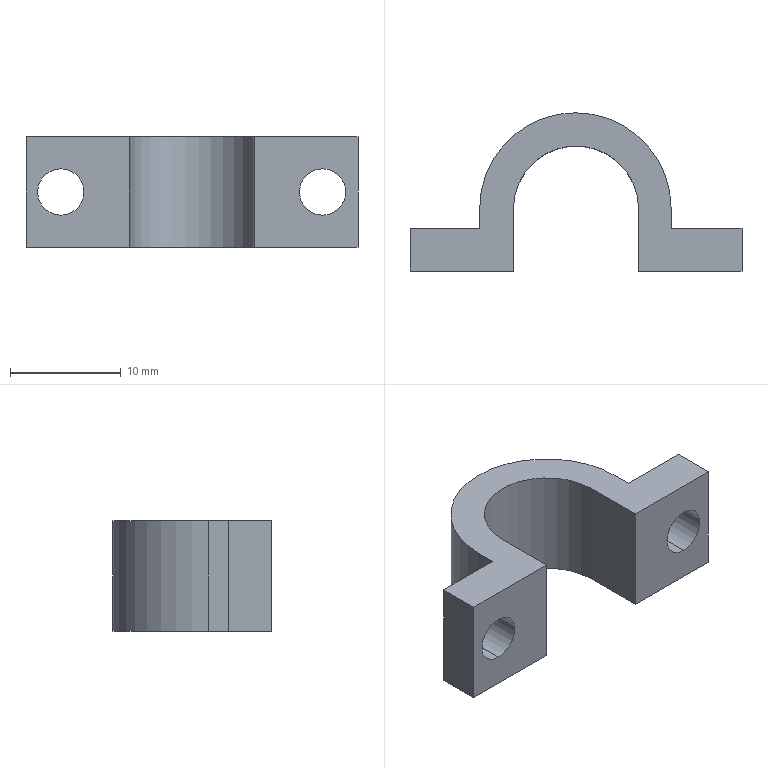Part | SolidWorks | features Cut 1, Extrusion 1 | 1 solid | 18 faces | box 30 x 14.3 x 10 mm | volume 1395 mm3 | plane 12 | cylinder 6 | commonest cylinder face diameters 4.2 x4 11.3 x1 17.3 x1
STEP:
#1=CARTESIAN_POINT('',(11.852,1.335,2.9));
#2=VERTEX_POINT('',#1);
#3=CARTESIAN_POINT('',(11.852,1.335,7.1));
#4=VERTEX_POINT('',#3);
#5=CARTESIAN_POINT('',(11.852,1.335,5.));
#6=DIRECTION('',(0.,1.,0.));
#7=DIRECTION('',(0.,0.,1.));
#8=AXIS2_PLACEMENT_3D('',#5,#6,#7);
#9=CIRCLE('',#8,2.1);
#10=EDGE_CURVE('',#2,#4,#9,.T.);
#11=ORIENTED_EDGE('',*,*,#10,.F.);
#12=CARTESIAN_POINT('',(11.852,5.185,2.9));
#13=VERTEX_POINT('',#12);
#14=CARTESIAN_POINT('',(11.852,-18.455,2.9));
#15=DIRECTION('',(0.,1.,0.));
#16=VECTOR('',#15,1000.);
#17=LINE('',#14,#16);
#18=EDGE_CURVE('',#2,#13,#17,.T.);
#19=ORIENTED_EDGE('',*,*,#18,.T.);
#20=CARTESIAN_POINT('',(11.852,5.185,7.1));
#21=VERTEX_POINT('',#20);
#22=CARTESIAN_POINT('',(11.852,5.185,5.));
#23=DIRECTION('',(0.,1.,0.));
#24=DIRECTION('',(0.,0.,1.));
#25=AXIS2_PLACEMENT_3D('',#22,#23,#24);
#26=CIRCLE('',#25,2.1);
#27=EDGE_CURVE('',#13,#21,#26,.T.);
#28=ORIENTED_EDGE('',*,*,#27,.T.);
#29=CARTESIAN_POINT('',(11.852,-18.455,7.1));
#30=DIRECTION('',(0.,1.,0.));
#31=VECTOR('',#30,1000.);
#32=LINE('',#29,#31);
#33=EDGE_CURVE('',#4,#21,#32,.T.);
#34=ORIENTED_EDGE('',*,*,#33,.F.);
#35=EDGE_LOOP('',(#11,#19,#28,#34));
#36=FACE_OUTER_BOUND('',#35,.T.);
#37=CARTESIAN_POINT('',(11.852,-18.455,5.));
#38=DIRECTION('',(0.,1.,0.));
#39=DIRECTION('',(0.,0.,1.));
#40=AXIS2_PLACEMENT_3D('',#37,#38,#39);
#41=CYLINDRICAL_SURFACE('',#40,2.1);
#42=ADVANCED_FACE('',(#36),#41,.F.);
#43=CARTESIAN_POINT('',(-11.798,1.335,2.9));
#44=VERTEX_POINT('',#43);
#45=CARTESIAN_POINT('',(-11.798,1.335,7.1));
#46=VERTEX_POINT('',#45);
#47=CARTESIAN_POINT('',(-11.798,1.335,5.));
#48=DIRECTION('',(0.,1.,0.));
#49=DIRECTION('',(0.,0.,1.));
#50=AXIS2_PLACEMENT_3D('',#47,#48,#49);
#51=CIRCLE('',#50,2.1);
#52=EDGE_CURVE('',#44,#46,#51,.T.);
#53=ORIENTED_EDGE('',*,*,#52,.F.);
#54=CARTESIAN_POINT('',(-11.798,5.185,2.9));
#55=VERTEX_POINT('',#54);
#56=CARTESIAN_POINT('',(-11.798,-18.455,2.9));
#57=DIRECTION('',(0.,1.,0.));
#58=VECTOR('',#57,1000.);
#59=LINE('',#56,#58);
#60=EDGE_CURVE('',#44,#55,#59,.T.);
#61=ORIENTED_EDGE('',*,*,#60,.T.);
#62=CARTESIAN_POINT('',(-11.798,5.185,7.1));
#63=VERTEX_POINT('',#62);
#64=CARTESIAN_POINT('',(-11.798,5.185,5.));
#65=DIRECTION('',(0.,1.,0.));
#66=DIRECTION('',(0.,0.,1.));
#67=AXIS2_PLACEMENT_3D('',#64,#65,#66);
#68=CIRCLE('',#67,2.1);
#69=EDGE_CURVE('',#55,#63,#68,.T.);
#70=ORIENTED_EDGE('',*,*,#69,.T.);
#71=CARTESIAN_POINT('',(-11.798,-18.455,7.1));
#72=DIRECTION('',(0.,1.,0.));
#73=VECTOR('',#72,1000.);
#74=LINE('',#71,#73);
#75=EDGE_CURVE('',#46,#63,#74,.T.);
#76=ORIENTED_EDGE('',*,*,#75,.F.);
#77=EDGE_LOOP('',(#53,#61,#70,#76));
#78=FACE_OUTER_BOUND('',#77,.T.);
#79=CARTESIAN_POINT('',(-11.798,-18.455,5.));
#80=DIRECTION('',(0.,1.,0.));
#81=DIRECTION('',(0.,0.,1.));
#82=AXIS2_PLACEMENT_3D('',#79,#80,#81);
#83=CYLINDRICAL_SURFACE('',#82,2.1);
#84=ADVANCED_FACE('',(#78),#83,.F.);
#85=CARTESIAN_POINT('',(-14.947,5.185,0.));
#86=VERTEX_POINT('',#85);
#87=CARTESIAN_POINT('',(-14.947,1.335,0.));
#88=VERTEX_POINT('',#87);
#89=CARTESIAN_POINT('',(-14.947,5.185,0.));
#90=DIRECTION('',(0.,-1.,0.));
#91=VECTOR('',#90,1000.);
#92=LINE('',#89,#91);
#93=EDGE_CURVE('',#86,#88,#92,.T.);
#94=ORIENTED_EDGE('',*,*,#93,.T.);
#95=CARTESIAN_POINT('',(-14.947,1.335,10.));
#96=VERTEX_POINT('',#95);
#97=CARTESIAN_POINT('',(-14.947,1.335,10.));
#98=DIRECTION('',(0.,0.,-1.));
#99=VECTOR('',#98,1000.);
#100=LINE('',#97,#99);
#101=EDGE_CURVE('',#96,#88,#100,.T.);
#102=ORIENTED_EDGE('',*,*,#101,.F.);
#103=CARTESIAN_POINT('',(-14.947,5.185,10.));
#104=VERTEX_POINT('',#103);
#105=CARTESIAN_POINT('',(-14.947,5.185,10.));
#106=DIRECTION('',(0.,-1.,0.));
#107=VECTOR('',#106,1000.);
#108=LINE('',#105,#107);
#109=EDGE_CURVE('',#104,#96,#108,.T.);
#110=ORIENTED_EDGE('',*,*,#109,.F.);
#111=CARTESIAN_POINT('',(-14.947,5.185,10.));
#112=DIRECTION('',(0.,0.,-1.));
#113=VECTOR('',#112,1000.);
#114=LINE('',#111,#113);
#115=EDGE_CURVE('',#104,#86,#114,.T.);
#116=ORIENTED_EDGE('',*,*,#115,.T.);
#117=EDGE_LOOP('',(#94,#102,#110,#116));
#118=FACE_OUTER_BOUND('',#117,.T.);
#119=CARTESIAN_POINT('',(-14.947,5.185,10.));
#120=DIRECTION('',(1.,0.,0.));
#121=DIRECTION('',(0.,0.,-1.));
#122=AXIS2_PLACEMENT_3D('',#119,#120,#121);
#123=PLANE('',#122);
#124=ADVANCED_FACE('',(#118),#123,.F.);
#125=CARTESIAN_POINT('',(-11.798,1.335,5.));
#126=DIRECTION('',(0.,1.,0.));
#127=DIRECTION('',(0.,0.,1.));
#128=AXIS2_PLACEMENT_3D('',#125,#126,#127);
#129=CIRCLE('',#128,2.1);
#130=EDGE_CURVE('',#46,#44,#129,.T.);
#131=ORIENTED_EDGE('',*,*,#130,.T.);
#132=ORIENTED_EDGE('',*,*,#52,.T.);
#133=EDGE_LOOP('',(#131,#132));
#134=FACE_BOUND('',#133,.T.);
#135=CARTESIAN_POINT('',(-5.597,1.335,0.));
#136=VERTEX_POINT('',#135);
#137=CARTESIAN_POINT('',(-14.947,1.335,0.));
#138=DIRECTION('',(1.,0.,0.));
#139=VECTOR('',#138,1000.);
#140=LINE('',#137,#139);
#141=EDGE_CURVE('',#88,#136,#140,.T.);
#142=ORIENTED_EDGE('',*,*,#141,.T.);
#143=CARTESIAN_POINT('',(-5.597,1.335,10.));
#144=VERTEX_POINT('',#143);
#145=CARTESIAN_POINT('',(-5.597,1.335,10.));
#146=DIRECTION('',(0.,0.,-1.));
#147=VECTOR('',#146,1000.);
#148=LINE('',#145,#147);
#149=EDGE_CURVE('',#144,#136,#148,.T.);
#150=ORIENTED_EDGE('',*,*,#149,.F.);
#151=CARTESIAN_POINT('',(-14.947,1.335,10.));
#152=DIRECTION('',(1.,0.,0.));
#153=VECTOR('',#152,1000.);
#154=LINE('',#151,#153);
#155=EDGE_CURVE('',#96,#144,#154,.T.);
#156=ORIENTED_EDGE('',*,*,#155,.F.);
#157=ORIENTED_EDGE('',*,*,#101,.T.);
#158=EDGE_LOOP('',(#142,#150,#156,#157));
#159=FACE_OUTER_BOUND('',#158,.T.);
#160=CARTESIAN_POINT('',(-14.947,1.335,10.));
#161=DIRECTION('',(0.,1.,0.));
#162=DIRECTION('',(0.,0.,1.));
#163=AXIS2_PLACEMENT_3D('',#160,#161,#162);
#164=PLANE('',#163);
#165=ADVANCED_FACE('',(#134,#159),#164,.F.);
#166=CARTESIAN_POINT('',(-5.597,6.985,0.));
#167=VERTEX_POINT('',#166);
#168=CARTESIAN_POINT('',(-5.597,5.185,0.));
#169=DIRECTION('',(0.,1.,0.));
#170=VECTOR('',#169,1000.);
#171=LINE('',#168,#170);
#172=EDGE_CURVE('',#136,#167,#171,.T.);
#173=ORIENTED_EDGE('',*,*,#172,.T.);
#174=CARTESIAN_POINT('',(-5.597,6.985,10.));
#175=VERTEX_POINT('',#174);
#176=CARTESIAN_POINT('',(-5.597,6.985,10.));
#177=DIRECTION('',(0.,0.,-1.));
#178=VECTOR('',#177,1000.);
#179=LINE('',#176,#178);
#180=EDGE_CURVE('',#175,#167,#179,.T.);
#181=ORIENTED_EDGE('',*,*,#180,.F.);
#182=CARTESIAN_POINT('',(-5.597,5.185,10.));
#183=DIRECTION('',(0.,1.,0.));
#184=VECTOR('',#183,1000.);
#185=LINE('',#182,#184);
#186=EDGE_CURVE('',#144,#175,#185,.T.);
#187=ORIENTED_EDGE('',*,*,#186,.F.);
#188=ORIENTED_EDGE('',*,*,#149,.T.);
#189=EDGE_LOOP('',(#173,#181,#187,#188));
#190=FACE_OUTER_BOUND('',#189,.T.);
#191=CARTESIAN_POINT('',(-5.597,5.185,10.));
#192=DIRECTION('',(-1.,0.,0.));
#193=DIRECTION('',(0.,0.,1.));
#194=AXIS2_PLACEMENT_3D('',#191,#192,#193);
#195=PLANE('',#194);
#196=ADVANCED_FACE('',(#190),#195,.F.);
#197=CARTESIAN_POINT('',(5.703,6.985,0.));
#198=VERTEX_POINT('',#197);
#199=CARTESIAN_POINT('',(0.05334,6.985,0.));
#200=DIRECTION('',(0.,0.,-1.));
#201=DIRECTION('',(1.,0.,0.));
#202=AXIS2_PLACEMENT_3D('',#199,#200,#201);
#203=CIRCLE('',#202,5.65);
#204=EDGE_CURVE('',#167,#198,#203,.T.);
#205=ORIENTED_EDGE('',*,*,#204,.T.);
#206=CARTESIAN_POINT('',(5.703,6.985,10.));
#207=VERTEX_POINT('',#206);
#208=CARTESIAN_POINT('',(5.703,6.985,10.));
#209=DIRECTION('',(0.,0.,-1.));
#210=VECTOR('',#209,1000.);
#211=LINE('',#208,#210);
#212=EDGE_CURVE('',#207,#198,#211,.T.);
#213=ORIENTED_EDGE('',*,*,#212,.F.);
#214=CARTESIAN_POINT('',(0.05334,6.985,10.));
#215=DIRECTION('',(0.,0.,-1.));
#216=DIRECTION('',(1.,0.,0.));
#217=AXIS2_PLACEMENT_3D('',#214,#215,#216);
#218=CIRCLE('',#217,5.65);
#219=EDGE_CURVE('',#175,#207,#218,.T.);
#220=ORIENTED_EDGE('',*,*,#219,.F.);
#221=ORIENTED_EDGE('',*,*,#180,.T.);
#222=EDGE_LOOP('',(#205,#213,#220,#221));
#223=FACE_OUTER_BOUND('',#222,.T.);
#224=CARTESIAN_POINT('',(0.05334,6.985,10.));
#225=DIRECTION('',(0.,0.,-1.));
#226=DIRECTION('',(-1.,0.,0.));
#227=AXIS2_PLACEMENT_3D('',#224,#225,#226);
#228=CYLINDRICAL_SURFACE('',#227,5.65);
#229=ADVANCED_FACE('',(#223),#228,.F.);
#230=CARTESIAN_POINT('',(5.703,1.335,0.));
#231=VERTEX_POINT('',#230);
#232=CARTESIAN_POINT('',(5.703,5.185,0.));
#233=DIRECTION('',(0.,-1.,0.));
#234=VECTOR('',#233,1000.);
#235=LINE('',#232,#234);
#236=EDGE_CURVE('',#198,#231,#235,.T.);
#237=ORIENTED_EDGE('',*,*,#236,.T.);
#238=CARTESIAN_POINT('',(5.703,1.335,10.));
#239=VERTEX_POINT('',#238);
#240=CARTESIAN_POINT('',(5.703,1.335,10.));
#241=DIRECTION('',(0.,0.,-1.));
#242=VECTOR('',#241,1000.);
#243=LINE('',#240,#242);
#244=EDGE_CURVE('',#239,#231,#243,.T.);
#245=ORIENTED_EDGE('',*,*,#244,.F.);
#246=CARTESIAN_POINT('',(5.703,6.985,10.));
#247=DIRECTION('',(0.,-1.,0.));
#248=VECTOR('',#247,1000.);
#249=LINE('',#246,#248);
#250=EDGE_CURVE('',#207,#239,#249,.T.);
#251=ORIENTED_EDGE('',*,*,#250,.F.);
#252=ORIENTED_EDGE('',*,*,#212,.T.);
#253=EDGE_LOOP('',(#237,#245,#251,#252));
#254=FACE_OUTER_BOUND('',#253,.T.);
#255=CARTESIAN_POINT('',(5.703,5.185,10.));
#256=DIRECTION('',(1.,0.,0.));
#257=DIRECTION('',(0.,1.,0.));
#258=AXIS2_PLACEMENT_3D('',#255,#256,#257);
#259=PLANE('',#258);
#260=ADVANCED_FACE('',(#254),#259,.F.);
#261=CARTESIAN_POINT('',(11.852,1.335,5.));
#262=DIRECTION('',(0.,1.,0.));
#263=DIRECTION('',(0.,0.,1.));
#264=AXIS2_PLACEMENT_3D('',#261,#262,#263);
#265=CIRCLE('',#264,2.1);
#266=EDGE_CURVE('',#4,#2,#265,.T.);
#267=ORIENTED_EDGE('',*,*,#266,.T.);
#268=ORIENTED_EDGE('',*,*,#10,.T.);
#269=EDGE_LOOP('',(#267,#268));
#270=FACE_BOUND('',#269,.T.);
#271=CARTESIAN_POINT('',(15.053,1.335,0.));
#272=VERTEX_POINT('',#271);
#273=CARTESIAN_POINT('',(5.703,1.335,0.));
#274=DIRECTION('',(1.,0.,0.));
#275=VECTOR('',#274,1000.);
#276=LINE('',#273,#275);
#277=EDGE_CURVE('',#231,#272,#276,.T.);
#278=ORIENTED_EDGE('',*,*,#277,.T.);
#279=CARTESIAN_POINT('',(15.053,1.335,10.));
#280=VERTEX_POINT('',#279);
#281=CARTESIAN_POINT('',(15.053,1.335,10.));
#282=DIRECTION('',(0.,0.,-1.));
#283=VECTOR('',#282,1000.);
#284=LINE('',#281,#283);
#285=EDGE_CURVE('',#280,#272,#284,.T.);
#286=ORIENTED_EDGE('',*,*,#285,.F.);
#287=CARTESIAN_POINT('',(5.703,1.335,10.));
#288=DIRECTION('',(1.,0.,0.));
#289=VECTOR('',#288,1000.);
#290=LINE('',#287,#289);
#291=EDGE_CURVE('',#239,#280,#290,.T.);
#292=ORIENTED_EDGE('',*,*,#291,.F.);
#293=ORIENTED_EDGE('',*,*,#244,.T.);
#294=EDGE_LOOP('',(#278,#286,#292,#293));
#295=FACE_OUTER_BOUND('',#294,.T.);
#296=CARTESIAN_POINT('',(5.703,1.335,10.));
#297=DIRECTION('',(0.,1.,0.));
#298=DIRECTION('',(0.,0.,1.));
#299=AXIS2_PLACEMENT_3D('',#296,#297,#298);
#300=PLANE('',#299);
#301=ADVANCED_FACE('',(#270,#295),#300,.F.);
#302=CARTESIAN_POINT('',(15.053,5.185,0.));
#303=VERTEX_POINT('',#302);
#304=CARTESIAN_POINT('',(15.053,5.185,0.));
#305=DIRECTION('',(0.,1.,0.));
#306=VECTOR('',#305,1000.);
#307=LINE('',#304,#306);
#308=EDGE_CURVE('',#272,#303,#307,.T.);
#309=ORIENTED_EDGE('',*,*,#308,.T.);
#310=CARTESIAN_POINT('',(15.053,5.185,10.));
#311=VERTEX_POINT('',#310);
#312=CARTESIAN_POINT('',(15.053,5.185,10.));
#313=DIRECTION('',(0.,0.,-1.));
#314=VECTOR('',#313,1000.);
#315=LINE('',#312,#314);
#316=EDGE_CURVE('',#311,#303,#315,.T.);
#317=ORIENTED_EDGE('',*,*,#316,.F.);
#318=CARTESIAN_POINT('',(15.053,5.185,10.));
#319=DIRECTION('',(0.,1.,0.));
#320=VECTOR('',#319,1000.);
#321=LINE('',#318,#320);
#322=EDGE_CURVE('',#280,#311,#321,.T.);
#323=ORIENTED_EDGE('',*,*,#322,.F.);
#324=ORIENTED_EDGE('',*,*,#285,.T.);
#325=EDGE_LOOP('',(#309,#317,#323,#324));
#326=FACE_OUTER_BOUND('',#325,.T.);
#327=CARTESIAN_POINT('',(15.053,5.185,10.));
#328=DIRECTION('',(-1.,0.,0.));
#329=DIRECTION('',(0.,-1.,0.));
#330=AXIS2_PLACEMENT_3D('',#327,#328,#329);
#331=PLANE('',#330);
#332=ADVANCED_FACE('',(#326),#331,.F.);
#333=CARTESIAN_POINT('',(11.852,5.185,5.));
#334=DIRECTION('',(0.,1.,0.));
#335=DIRECTION('',(0.,0.,1.));
#336=AXIS2_PLACEMENT_3D('',#333,#334,#335);
#337=CIRCLE('',#336,2.1);
#338=EDGE_CURVE('',#21,#13,#337,.T.);
#339=ORIENTED_EDGE('',*,*,#338,.F.);
#340=ORIENTED_EDGE('',*,*,#27,.F.);
#341=EDGE_LOOP('',(#339,#340));
#342=FACE_BOUND('',#341,.T.);
#343=CARTESIAN_POINT('',(8.65,5.185,0.));
#344=VERTEX_POINT('',#343);
#345=CARTESIAN_POINT('',(8.65,5.185,0.));
#346=DIRECTION('',(-1.,0.,0.));
#347=VECTOR('',#346,1000.);
#348=LINE('',#345,#347);
#349=EDGE_CURVE('',#303,#344,#348,.T.);
#350=ORIENTED_EDGE('',*,*,#349,.T.);
#351=CARTESIAN_POINT('',(8.65,5.185,10.));
#352=VERTEX_POINT('',#351);
#353=CARTESIAN_POINT('',(8.65,5.185,10.));
#354=DIRECTION('',(0.,0.,-1.));
#355=VECTOR('',#354,1000.);
#356=LINE('',#353,#355);
#357=EDGE_CURVE('',#352,#344,#356,.T.);
#358=ORIENTED_EDGE('',*,*,#357,.F.);
#359=CARTESIAN_POINT('',(8.65,5.185,10.));
#360=DIRECTION('',(-1.,0.,0.));
#361=VECTOR('',#360,1000.);
#362=LINE('',#359,#361);
#363=EDGE_CURVE('',#311,#352,#362,.T.);
#364=ORIENTED_EDGE('',*,*,#363,.F.);
#365=ORIENTED_EDGE('',*,*,#316,.T.);
#366=EDGE_LOOP('',(#350,#358,#364,#365));
#367=FACE_OUTER_BOUND('',#366,.T.);
#368=CARTESIAN_POINT('',(8.65,5.185,10.));
#369=DIRECTION('',(0.,-1.,0.));
#370=DIRECTION('',(0.,0.,-1.));
#371=AXIS2_PLACEMENT_3D('',#368,#369,#370);
#372=PLANE('',#371);
#373=ADVANCED_FACE('',(#342,#367),#372,.F.);
#374=CARTESIAN_POINT('',(8.65,6.985,0.));
#375=VERTEX_POINT('',#374);
#376=CARTESIAN_POINT('',(8.65,6.985,0.));
#377=DIRECTION('',(0.,1.,0.));
#378=VECTOR('',#377,1000.);
#379=LINE('',#376,#378);
#380=EDGE_CURVE('',#344,#375,#379,.T.);
#381=ORIENTED_EDGE('',*,*,#380,.T.);
#382=CARTESIAN_POINT('',(8.65,6.985,10.));
#383=VERTEX_POINT('',#382);
#384=CARTESIAN_POINT('',(8.65,6.985,10.));
#385=DIRECTION('',(0.,0.,-1.));
#386=VECTOR('',#385,1000.);
#387=LINE('',#384,#386);
#388=EDGE_CURVE('',#383,#375,#387,.T.);
#389=ORIENTED_EDGE('',*,*,#388,.F.);
#390=CARTESIAN_POINT('',(8.65,6.985,10.));
#391=DIRECTION('',(0.,1.,0.));
#392=VECTOR('',#391,1000.);
#393=LINE('',#390,#392);
#394=EDGE_CURVE('',#352,#383,#393,.T.);
#395=ORIENTED_EDGE('',*,*,#394,.F.);
#396=ORIENTED_EDGE('',*,*,#357,.T.);
#397=EDGE_LOOP('',(#381,#389,#395,#396));
#398=FACE_OUTER_BOUND('',#397,.T.);
#399=CARTESIAN_POINT('',(8.65,6.985,10.));
#400=DIRECTION('',(-1.,0.,0.));
#401=DIRECTION('',(0.,0.,1.));
#402=AXIS2_PLACEMENT_3D('',#399,#400,#401);
#403=PLANE('',#402);
#404=ADVANCED_FACE('',(#398),#403,.F.);
#405=CARTESIAN_POINT('',(-8.65,6.985,0.));
#406=VERTEX_POINT('',#405);
#407=CARTESIAN_POINT('',(0.,6.985,0.));
#408=DIRECTION('',(0.,0.,1.));
#409=DIRECTION('',(1.,0.,0.));
#410=AXIS2_PLACEMENT_3D('',#407,#408,#409);
#411=CIRCLE('',#410,8.65);
#412=EDGE_CURVE('',#375,#406,#411,.T.);
#413=ORIENTED_EDGE('',*,*,#412,.T.);
#414=CARTESIAN_POINT('',(-8.65,6.985,10.));
#415=VERTEX_POINT('',#414);
#416=CARTESIAN_POINT('',(-8.65,6.985,10.));
#417=DIRECTION('',(0.,0.,-1.));
#418=VECTOR('',#417,1000.);
#419=LINE('',#416,#418);
#420=EDGE_CURVE('',#415,#406,#419,.T.);
#421=ORIENTED_EDGE('',*,*,#420,.F.);
#422=CARTESIAN_POINT('',(0.,6.985,10.));
#423=DIRECTION('',(0.,0.,1.));
#424=DIRECTION('',(1.,0.,0.));
#425=AXIS2_PLACEMENT_3D('',#422,#423,#424);
#426=CIRCLE('',#425,8.65);
#427=EDGE_CURVE('',#383,#415,#426,.T.);
#428=ORIENTED_EDGE('',*,*,#427,.F.);
#429=ORIENTED_EDGE('',*,*,#388,.T.);
#430=EDGE_LOOP('',(#413,#421,#428,#429));
#431=FACE_OUTER_BOUND('',#430,.T.);
#432=CARTESIAN_POINT('',(0.,6.985,10.));
#433=DIRECTION('',(0.,0.,-1.));
#434=DIRECTION('',(-1.,0.,0.));
#435=AXIS2_PLACEMENT_3D('',#432,#433,#434);
#436=CYLINDRICAL_SURFACE('',#435,8.65);
#437=ADVANCED_FACE('',(#431),#436,.T.);
#438=CARTESIAN_POINT('',(-8.65,5.185,0.));
#439=VERTEX_POINT('',#438);
#440=CARTESIAN_POINT('',(-8.65,6.985,0.));
#441=DIRECTION('',(0.,-1.,0.));
#442=VECTOR('',#441,1000.);
#443=LINE('',#440,#442);
#444=EDGE_CURVE('',#406,#439,#443,.T.);
#445=ORIENTED_EDGE('',*,*,#444,.T.);
#446=CARTESIAN_POINT('',(-8.65,5.185,10.));
#447=VERTEX_POINT('',#446);
#448=CARTESIAN_POINT('',(-8.65,5.185,10.));
#449=DIRECTION('',(0.,0.,-1.));
#450=VECTOR('',#449,1000.);
#451=LINE('',#448,#450);
#452=EDGE_CURVE('',#447,#439,#451,.T.);
#453=ORIENTED_EDGE('',*,*,#452,.F.);
#454=CARTESIAN_POINT('',(-8.65,6.985,10.));
#455=DIRECTION('',(0.,-1.,0.));
#456=VECTOR('',#455,1000.);
#457=LINE('',#454,#456);
#458=EDGE_CURVE('',#415,#447,#457,.T.);
#459=ORIENTED_EDGE('',*,*,#458,.F.);
#460=ORIENTED_EDGE('',*,*,#420,.T.);
#461=EDGE_LOOP('',(#445,#453,#459,#460));
#462=FACE_OUTER_BOUND('',#461,.T.);
#463=CARTESIAN_POINT('',(-8.65,6.985,10.));
#464=DIRECTION('',(1.,0.,0.));
#465=DIRECTION('',(0.,0.,-1.));
#466=AXIS2_PLACEMENT_3D('',#463,#464,#465);
#467=PLANE('',#466);
#468=ADVANCED_FACE('',(#462),#467,.F.);
#469=CARTESIAN_POINT('',(-11.798,5.185,5.));
#470=DIRECTION('',(0.,1.,0.));
#471=DIRECTION('',(0.,0.,1.));
#472=AXIS2_PLACEMENT_3D('',#469,#470,#471);
#473=CIRCLE('',#472,2.1);
#474=EDGE_CURVE('',#63,#55,#473,.T.);
#475=ORIENTED_EDGE('',*,*,#474,.F.);
#476=ORIENTED_EDGE('',*,*,#69,.F.);
#477=EDGE_LOOP('',(#475,#476));
#478=FACE_BOUND('',#477,.T.);
#479=CARTESIAN_POINT('',(-14.947,5.185,0.));
#480=DIRECTION('',(-1.,0.,0.));
#481=VECTOR('',#480,1000.);
#482=LINE('',#479,#481);
#483=EDGE_CURVE('',#439,#86,#482,.T.);
#484=ORIENTED_EDGE('',*,*,#483,.T.);
#485=ORIENTED_EDGE('',*,*,#115,.F.);
#486=CARTESIAN_POINT('',(-14.947,5.185,10.));
#487=DIRECTION('',(-1.,0.,0.));
#488=VECTOR('',#487,1000.);
#489=LINE('',#486,#488);
#490=EDGE_CURVE('',#447,#104,#489,.T.);
#491=ORIENTED_EDGE('',*,*,#490,.F.);
#492=ORIENTED_EDGE('',*,*,#452,.T.);
#493=EDGE_LOOP('',(#484,#485,#491,#492));
#494=FACE_OUTER_BOUND('',#493,.T.);
#495=CARTESIAN_POINT('',(-14.947,5.185,10.));
#496=DIRECTION('',(0.,-1.,0.));
#497=DIRECTION('',(0.,0.,-1.));
#498=AXIS2_PLACEMENT_3D('',#495,#496,#497);
#499=PLANE('',#498);
#500=ADVANCED_FACE('',(#478,#494),#499,.F.);
#501=ORIENTED_EDGE('',*,*,#109,.T.);
#502=ORIENTED_EDGE('',*,*,#155,.T.);
#503=ORIENTED_EDGE('',*,*,#186,.T.);
#504=ORIENTED_EDGE('',*,*,#219,.T.);
#505=ORIENTED_EDGE('',*,*,#250,.T.);
#506=ORIENTED_EDGE('',*,*,#291,.T.);
#507=ORIENTED_EDGE('',*,*,#322,.T.);
#508=ORIENTED_EDGE('',*,*,#363,.T.);
#509=ORIENTED_EDGE('',*,*,#394,.T.);
#510=ORIENTED_EDGE('',*,*,#427,.T.);
#511=ORIENTED_EDGE('',*,*,#458,.T.);
#512=ORIENTED_EDGE('',*,*,#490,.T.);
#513=EDGE_LOOP('',(#501,#502,#503,#504,#505,#506,#507,#508,#509,#510,#511,#512));
#514=FACE_OUTER_BOUND('',#513,.T.);
#515=CARTESIAN_POINT('',(0.05334,6.985,10.));
#516=DIRECTION('',(0.,0.,1.));
#517=DIRECTION('',(1.,0.,0.));
#518=AXIS2_PLACEMENT_3D('',#515,#516,#517);
#519=PLANE('',#518);
#520=ADVANCED_FACE('',(#514),#519,.T.);
#521=ORIENTED_EDGE('',*,*,#93,.F.);
#522=ORIENTED_EDGE('',*,*,#483,.F.);
#523=ORIENTED_EDGE('',*,*,#444,.F.);
#524=ORIENTED_EDGE('',*,*,#412,.F.);
#525=ORIENTED_EDGE('',*,*,#380,.F.);
#526=ORIENTED_EDGE('',*,*,#349,.F.);
#527=ORIENTED_EDGE('',*,*,#308,.F.);
#528=ORIENTED_EDGE('',*,*,#277,.F.);
#529=ORIENTED_EDGE('',*,*,#236,.F.);
#530=ORIENTED_EDGE('',*,*,#204,.F.);
#531=ORIENTED_EDGE('',*,*,#172,.F.);
#532=ORIENTED_EDGE('',*,*,#141,.F.);
#533=EDGE_LOOP('',(#521,#522,#523,#524,#525,#526,#527,#528,#529,#530,#531,#532));
#534=FACE_OUTER_BOUND('',#533,.T.);
#535=CARTESIAN_POINT('',(0.05334,6.985,0.));
#536=DIRECTION('',(0.,0.,1.));
#537=DIRECTION('',(1.,0.,0.));
#538=AXIS2_PLACEMENT_3D('',#535,#536,#537);
#539=PLANE('',#538);
#540=ADVANCED_FACE('',(#534),#539,.F.);
#541=ORIENTED_EDGE('',*,*,#60,.F.);
#542=ORIENTED_EDGE('',*,*,#130,.F.);
#543=ORIENTED_EDGE('',*,*,#75,.T.);
#544=ORIENTED_EDGE('',*,*,#474,.T.);
#545=EDGE_LOOP('',(#541,#542,#543,#544));
#546=FACE_OUTER_BOUND('',#545,.T.);
#547=CARTESIAN_POINT('',(-11.798,-18.455,5.));
#548=DIRECTION('',(0.,1.,0.));
#549=DIRECTION('',(0.,0.,1.));
#550=AXIS2_PLACEMENT_3D('',#547,#548,#549);
#551=CYLINDRICAL_SURFACE('',#550,2.1);
#552=ADVANCED_FACE('',(#546),#551,.F.);
#553=ORIENTED_EDGE('',*,*,#18,.F.);
#554=ORIENTED_EDGE('',*,*,#266,.F.);
#555=ORIENTED_EDGE('',*,*,#33,.T.);
#556=ORIENTED_EDGE('',*,*,#338,.T.);
#557=EDGE_LOOP('',(#553,#554,#555,#556));
#558=FACE_OUTER_BOUND('',#557,.T.);
#559=CARTESIAN_POINT('',(11.852,-18.455,5.));
#560=DIRECTION('',(0.,1.,0.));
#561=DIRECTION('',(0.,0.,1.));
#562=AXIS2_PLACEMENT_3D('',#559,#560,#561);
#563=CYLINDRICAL_SURFACE('',#562,2.1);
#564=ADVANCED_FACE('',(#558),#563,.F.);
#565=CLOSED_SHELL('',(#42,#84,#124,#165,#196,#229,#260,#301,#332,#373,#404,#437,#468,#500,#520,#540,#552,#564));
#566=MANIFOLD_SOLID_BREP('',#565);
#567=CARTESIAN_POINT('',(0.,0.,0.));
#568=DIRECTION('',(0.,0.,1.));
#569=DIRECTION('',(1.,0.,0.));
#570=AXIS2_PLACEMENT_3D('',#567,#568,#569);
#571=(LENGTH_UNIT()NAMED_UNIT(*)SI_UNIT(.MILLI.,.METRE.));
#572=UNCERTAINTY_MEASURE_WITH_UNIT(LENGTH_MEASURE(0.00001),#571,'','');
#573=(NAMED_UNIT(*)PLANE_ANGLE_UNIT()SI_UNIT($,.RADIAN.));
#574=(NAMED_UNIT(*)SI_UNIT($,.STERADIAN.)SOLID_ANGLE_UNIT());
#575=(GEOMETRIC_REPRESENTATION_CONTEXT(3)GLOBAL_UNCERTAINTY_ASSIGNED_CONTEXT((#572))GLOBAL_UNIT_ASSIGNED_CONTEXT((#571,#573,#574))REPRESENTATION_CONTEXT('',''));
#576=ADVANCED_BREP_SHAPE_REPRESENTATION('',(#566,#570),#575);